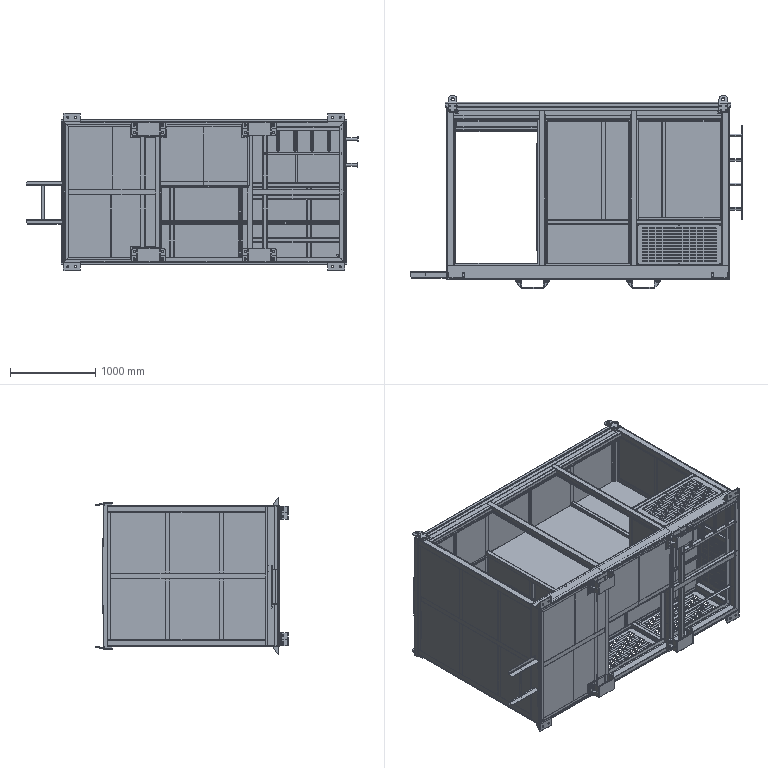Part | SolidWorks | 425 solids | 12634 faces | volume 198601111 mm3 | plane 7372 | cylinder 4526 | cone 384 | spline 352 | commonest cylinder face diameters 15 x1008 6 x686 10 x446 0.2 x386 9 x295 12 x212